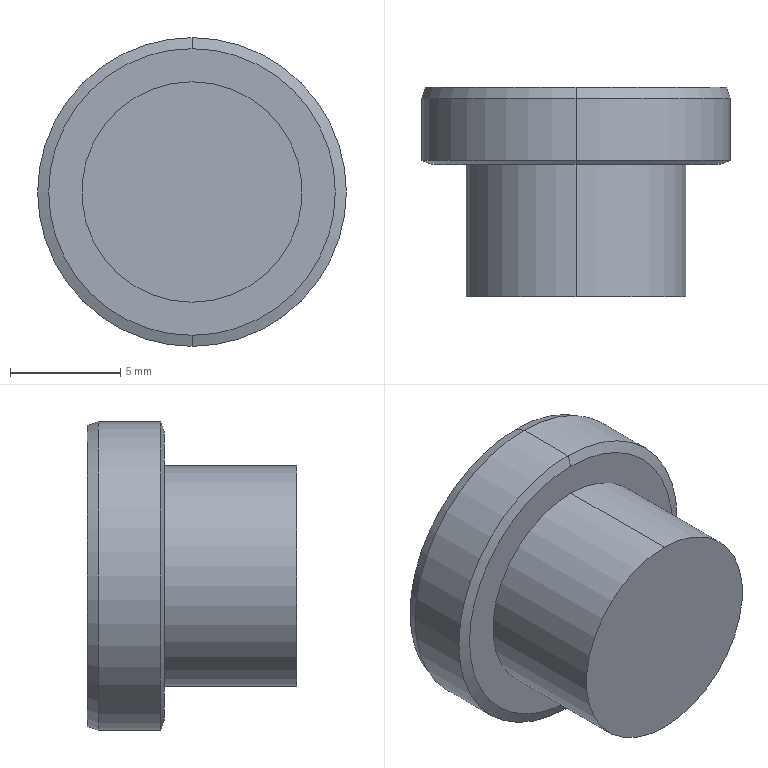Part | SolidWorks | features ICE 2, Chamfer 1, Extrusion 1 | 1 solid | 18 faces | box 14 x 9.5 x 14 mm | volume 897.832 mm3 | plane 10 | cone 4 | cylinder 4 | commonest cylinder face diameters 10 x2 14 x2
STEP:
#1=CARTESIAN_POINT('',(0.,9.5,6.818));
#2=VERTEX_POINT('',#1);
#3=CARTESIAN_POINT('',(0.,9.5,-6.818));
#4=VERTEX_POINT('',#3);
#5=CARTESIAN_POINT('',(0.,9.5,0.));
#6=DIRECTION('',(0.,1.,0.));
#7=DIRECTION('',(0.,0.,1.));
#8=AXIS2_PLACEMENT_3D('',#5,#6,#7);
#9=CIRCLE('',#8,6.818);
#10=EDGE_CURVE('',#2,#4,#9,.T.);
#11=ORIENTED_EDGE('',*,*,#10,.F.);
#12=CARTESIAN_POINT('',(0.,9.,7.));
#13=VERTEX_POINT('',#12);
#14=CARTESIAN_POINT('',(0.,9.5,6.818));
#15=DIRECTION('',(0.,-0.9397,0.342));
#16=VECTOR('',#15,1000.);
#17=LINE('',#14,#16);
#18=EDGE_CURVE('',#2,#13,#17,.T.);
#19=ORIENTED_EDGE('',*,*,#18,.T.);
#20=CARTESIAN_POINT('',(0.,9.,-7.));
#21=VERTEX_POINT('',#20);
#22=CARTESIAN_POINT('',(0.,9.,0.));
#23=DIRECTION('',(0.,-1.,0.));
#24=DIRECTION('',(0.,0.,1.));
#25=AXIS2_PLACEMENT_3D('',#22,#23,#24);
#26=CIRCLE('',#25,7.);
#27=EDGE_CURVE('',#21,#13,#26,.T.);
#28=ORIENTED_EDGE('',*,*,#27,.F.);
#29=CARTESIAN_POINT('',(0.,9.5,-6.818));
#30=DIRECTION('',(0.,-0.9397,-0.342));
#31=VECTOR('',#30,1000.);
#32=LINE('',#29,#31);
#33=EDGE_CURVE('',#4,#21,#32,.T.);
#34=ORIENTED_EDGE('',*,*,#33,.F.);
#35=EDGE_LOOP('',(#11,#19,#28,#34));
#36=FACE_OUTER_BOUND('',#35,.T.);
#37=CARTESIAN_POINT('',(0.,9.5,0.));
#38=DIRECTION('',(0.,-1.,0.));
#39=DIRECTION('',(0.,0.,-1.));
#40=AXIS2_PLACEMENT_3D('',#37,#38,#39);
#41=CONICAL_SURFACE('',#40,6.818,0.3491);
#42=ADVANCED_FACE('',(#36),#41,.T.);
#43=CARTESIAN_POINT('',(0.,6.,-6.5));
#44=VERTEX_POINT('',#43);
#45=CARTESIAN_POINT('',(0.,6.,6.5));
#46=VERTEX_POINT('',#45);
#47=CARTESIAN_POINT('',(0.,6.,0.));
#48=DIRECTION('',(0.,-1.,0.));
#49=DIRECTION('',(0.,0.,1.));
#50=AXIS2_PLACEMENT_3D('',#47,#48,#49);
#51=CIRCLE('',#50,6.5);
#52=EDGE_CURVE('',#44,#46,#51,.T.);
#53=ORIENTED_EDGE('',*,*,#52,.F.);
#54=CARTESIAN_POINT('',(0.,6.182,-7.));
#55=VERTEX_POINT('',#54);
#56=CARTESIAN_POINT('',(0.,6.182,-7.));
#57=DIRECTION('',(0.,0.342,-0.9397));
#58=VECTOR('',#57,1000.);
#59=LINE('',#56,#58);
#60=EDGE_CURVE('',#44,#55,#59,.T.);
#61=ORIENTED_EDGE('',*,*,#60,.T.);
#62=CARTESIAN_POINT('',(0.,6.182,7.));
#63=VERTEX_POINT('',#62);
#64=CARTESIAN_POINT('',(0.,6.182,0.));
#65=DIRECTION('',(0.,1.,0.));
#66=DIRECTION('',(0.,0.,1.));
#67=AXIS2_PLACEMENT_3D('',#64,#65,#66);
#68=CIRCLE('',#67,7.);
#69=EDGE_CURVE('',#63,#55,#68,.T.);
#70=ORIENTED_EDGE('',*,*,#69,.F.);
#71=CARTESIAN_POINT('',(0.,6.182,7.));
#72=DIRECTION('',(0.,0.342,0.9397));
#73=VECTOR('',#72,1000.);
#74=LINE('',#71,#73);
#75=EDGE_CURVE('',#46,#63,#74,.T.);
#76=ORIENTED_EDGE('',*,*,#75,.F.);
#77=EDGE_LOOP('',(#53,#61,#70,#76));
#78=FACE_OUTER_BOUND('',#77,.T.);
#79=CARTESIAN_POINT('',(0.,6.182,0.));
#80=DIRECTION('',(0.,1.,0.));
#81=DIRECTION('',(0.,0.,1.));
#82=AXIS2_PLACEMENT_3D('',#79,#80,#81);
#83=CONICAL_SURFACE('',#82,7.,1.222);
#84=ADVANCED_FACE('',(#78),#83,.T.);
#85=ORIENTED_EDGE('',*,*,#27,.T.);
#86=CARTESIAN_POINT('',(0.,9.5,7.));
#87=DIRECTION('',(0.,-1.,0.));
#88=VECTOR('',#87,1000.);
#89=LINE('',#86,#88);
#90=EDGE_CURVE('',#13,#63,#89,.T.);
#91=ORIENTED_EDGE('',*,*,#90,.T.);
#92=ORIENTED_EDGE('',*,*,#69,.T.);
#93=CARTESIAN_POINT('',(0.,9.5,-7.));
#94=DIRECTION('',(0.,-1.,0.));
#95=VECTOR('',#94,1000.);
#96=LINE('',#93,#95);
#97=EDGE_CURVE('',#21,#55,#96,.T.);
#98=ORIENTED_EDGE('',*,*,#97,.F.);
#99=EDGE_LOOP('',(#85,#91,#92,#98));
#100=FACE_OUTER_BOUND('',#99,.T.);
#101=CARTESIAN_POINT('',(0.,9.5,0.));
#102=DIRECTION('',(0.,-1.,0.));
#103=DIRECTION('',(0.,0.,-1.));
#104=AXIS2_PLACEMENT_3D('',#101,#102,#103);
#105=CYLINDRICAL_SURFACE('',#104,7.);
#106=ADVANCED_FACE('',(#100),#105,.T.);
#107=CARTESIAN_POINT('',(0.,6.,5.));
#108=VERTEX_POINT('',#107);
#109=CARTESIAN_POINT('',(0.,6.,-5.));
#110=VERTEX_POINT('',#109);
#111=CARTESIAN_POINT('',(0.,6.,0.));
#112=DIRECTION('',(0.,1.,0.));
#113=DIRECTION('',(0.,0.,1.));
#114=AXIS2_PLACEMENT_3D('',#111,#112,#113);
#115=CIRCLE('',#114,5.);
#116=EDGE_CURVE('',#108,#110,#115,.T.);
#117=ORIENTED_EDGE('',*,*,#116,.F.);
#118=CARTESIAN_POINT('',(0.,0.,5.));
#119=VERTEX_POINT('',#118);
#120=CARTESIAN_POINT('',(0.,6.,5.));
#121=DIRECTION('',(0.,-1.,0.));
#122=VECTOR('',#121,1000.);
#123=LINE('',#120,#122);
#124=EDGE_CURVE('',#108,#119,#123,.T.);
#125=ORIENTED_EDGE('',*,*,#124,.T.);
#126=CARTESIAN_POINT('',(0.,0.,-5.));
#127=VERTEX_POINT('',#126);
#128=CARTESIAN_POINT('',(0.,0.,0.));
#129=DIRECTION('',(0.,1.,0.));
#130=DIRECTION('',(0.,0.,1.));
#131=AXIS2_PLACEMENT_3D('',#128,#129,#130);
#132=CIRCLE('',#131,5.);
#133=EDGE_CURVE('',#119,#127,#132,.T.);
#134=ORIENTED_EDGE('',*,*,#133,.T.);
#135=CARTESIAN_POINT('',(0.,6.,-5.));
#136=DIRECTION('',(0.,-1.,0.));
#137=VECTOR('',#136,1000.);
#138=LINE('',#135,#137);
#139=EDGE_CURVE('',#110,#127,#138,.T.);
#140=ORIENTED_EDGE('',*,*,#139,.F.);
#141=EDGE_LOOP('',(#117,#125,#134,#140));
#142=FACE_OUTER_BOUND('',#141,.T.);
#143=CARTESIAN_POINT('',(0.,6.,0.));
#144=DIRECTION('',(0.,-1.,0.));
#145=DIRECTION('',(0.,0.,-1.));
#146=AXIS2_PLACEMENT_3D('',#143,#144,#145);
#147=CYLINDRICAL_SURFACE('',#146,5.);
#148=ADVANCED_FACE('',(#142),#147,.T.);
#149=ORIENTED_EDGE('',*,*,#124,.F.);
#150=CARTESIAN_POINT('',(0.,6.,0.));
#151=DIRECTION('',(0.,1.,0.));
#152=DIRECTION('',(0.,0.,1.));
#153=AXIS2_PLACEMENT_3D('',#150,#151,#152);
#154=CIRCLE('',#153,5.);
#155=EDGE_CURVE('',#110,#108,#154,.T.);
#156=ORIENTED_EDGE('',*,*,#155,.F.);
#157=ORIENTED_EDGE('',*,*,#139,.T.);
#158=CARTESIAN_POINT('',(0.,0.,0.));
#159=DIRECTION('',(0.,1.,0.));
#160=DIRECTION('',(0.,0.,1.));
#161=AXIS2_PLACEMENT_3D('',#158,#159,#160);
#162=CIRCLE('',#161,5.);
#163=EDGE_CURVE('',#127,#119,#162,.T.);
#164=ORIENTED_EDGE('',*,*,#163,.T.);
#165=EDGE_LOOP('',(#149,#156,#157,#164));
#166=FACE_OUTER_BOUND('',#165,.T.);
#167=CARTESIAN_POINT('',(0.,6.,0.));
#168=DIRECTION('',(0.,-1.,0.));
#169=DIRECTION('',(0.,0.,-1.));
#170=AXIS2_PLACEMENT_3D('',#167,#168,#169);
#171=CYLINDRICAL_SURFACE('',#170,5.);
#172=ADVANCED_FACE('',(#166),#171,.T.);
#173=ORIENTED_EDGE('',*,*,#163,.F.);
#174=ORIENTED_EDGE('',*,*,#133,.F.);
#175=EDGE_LOOP('',(#173,#174));
#176=FACE_OUTER_BOUND('',#175,.T.);
#177=CARTESIAN_POINT('',(0.,0.,0.));
#178=DIRECTION('',(0.,1.,0.));
#179=DIRECTION('',(0.,0.,1.));
#180=AXIS2_PLACEMENT_3D('',#177,#178,#179);
#181=PLANE('',#180);
#182=ADVANCED_FACE('',(#176),#181,.F.);
#183=ORIENTED_EDGE('',*,*,#90,.F.);
#184=CARTESIAN_POINT('',(0.,9.,0.));
#185=DIRECTION('',(0.,-1.,0.));
#186=DIRECTION('',(0.,0.,1.));
#187=AXIS2_PLACEMENT_3D('',#184,#185,#186);
#188=CIRCLE('',#187,7.);
#189=EDGE_CURVE('',#13,#21,#188,.T.);
#190=ORIENTED_EDGE('',*,*,#189,.T.);
#191=ORIENTED_EDGE('',*,*,#97,.T.);
#192=CARTESIAN_POINT('',(0.,6.182,0.));
#193=DIRECTION('',(0.,1.,0.));
#194=DIRECTION('',(0.,0.,1.));
#195=AXIS2_PLACEMENT_3D('',#192,#193,#194);
#196=CIRCLE('',#195,7.);
#197=EDGE_CURVE('',#55,#63,#196,.T.);
#198=ORIENTED_EDGE('',*,*,#197,.T.);
#199=EDGE_LOOP('',(#183,#190,#191,#198));
#200=FACE_OUTER_BOUND('',#199,.T.);
#201=CARTESIAN_POINT('',(0.,9.5,0.));
#202=DIRECTION('',(0.,-1.,0.));
#203=DIRECTION('',(0.,0.,-1.));
#204=AXIS2_PLACEMENT_3D('',#201,#202,#203);
#205=CYLINDRICAL_SURFACE('',#204,7.);
#206=ADVANCED_FACE('',(#200),#205,.T.);
#207=CARTESIAN_POINT('',(0.,9.5,0.));
#208=DIRECTION('',(0.,1.,0.));
#209=DIRECTION('',(0.,0.,1.));
#210=AXIS2_PLACEMENT_3D('',#207,#208,#209);
#211=CIRCLE('',#210,6.818);
#212=EDGE_CURVE('',#4,#2,#211,.T.);
#213=ORIENTED_EDGE('',*,*,#212,.T.);
#214=ORIENTED_EDGE('',*,*,#10,.T.);
#215=EDGE_LOOP('',(#213,#214));
#216=FACE_OUTER_BOUND('',#215,.T.);
#217=CARTESIAN_POINT('',(-1.443,9.5,-2.5));
#218=VERTEX_POINT('',#217);
#219=CARTESIAN_POINT('',(-2.887,9.5,0.));
#220=VERTEX_POINT('',#219);
#221=CARTESIAN_POINT('',(-1.443,9.5,-2.5));
#222=DIRECTION('',(-0.5,0.,0.866));
#223=VECTOR('',#222,1000.);
#224=LINE('',#221,#223);
#225=EDGE_CURVE('',#218,#220,#224,.T.);
#226=ORIENTED_EDGE('',*,*,#225,.F.);
#227=CARTESIAN_POINT('',(1.443,9.5,-2.5));
#228=VERTEX_POINT('',#227);
#229=CARTESIAN_POINT('',(1.443,9.5,-2.5));
#230=DIRECTION('',(-1.,0.,0.));
#231=VECTOR('',#230,1000.);
#232=LINE('',#229,#231);
#233=EDGE_CURVE('',#228,#218,#232,.T.);
#234=ORIENTED_EDGE('',*,*,#233,.F.);
#235=CARTESIAN_POINT('',(2.887,9.5,0.));
#236=VERTEX_POINT('',#235);
#237=CARTESIAN_POINT('',(2.887,9.5,0.));
#238=DIRECTION('',(-0.5,0.,-0.866));
#239=VECTOR('',#238,1000.);
#240=LINE('',#237,#239);
#241=EDGE_CURVE('',#236,#228,#240,.T.);
#242=ORIENTED_EDGE('',*,*,#241,.F.);
#243=CARTESIAN_POINT('',(1.443,9.5,2.5));
#244=VERTEX_POINT('',#243);
#245=CARTESIAN_POINT('',(1.443,9.5,2.5));
#246=DIRECTION('',(0.5,0.,-0.866));
#247=VECTOR('',#246,1000.);
#248=LINE('',#245,#247);
#249=EDGE_CURVE('',#244,#236,#248,.T.);
#250=ORIENTED_EDGE('',*,*,#249,.F.);
#251=CARTESIAN_POINT('',(-1.443,9.5,2.5));
#252=VERTEX_POINT('',#251);
#253=CARTESIAN_POINT('',(-1.443,9.5,2.5));
#254=DIRECTION('',(1.,0.,0.));
#255=VECTOR('',#254,1000.);
#256=LINE('',#253,#255);
#257=EDGE_CURVE('',#252,#244,#256,.T.);
#258=ORIENTED_EDGE('',*,*,#257,.F.);
#259=CARTESIAN_POINT('',(-2.887,9.5,0.));
#260=DIRECTION('',(0.5,0.,0.866));
#261=VECTOR('',#260,1000.);
#262=LINE('',#259,#261);
#263=EDGE_CURVE('',#220,#252,#262,.T.);
#264=ORIENTED_EDGE('',*,*,#263,.F.);
#265=EDGE_LOOP('',(#226,#234,#242,#250,#258,#264));
#266=FACE_BOUND('',#265,.T.);
#267=CARTESIAN_POINT('',(0.,9.5,0.));
#268=DIRECTION('',(0.,1.,0.));
#269=DIRECTION('',(0.,0.,1.));
#270=AXIS2_PLACEMENT_3D('',#267,#268,#269);
#271=PLANE('',#270);
#272=ADVANCED_FACE('',(#216,#266),#271,.T.);
#273=CARTESIAN_POINT('',(0.,6.,0.));
#274=DIRECTION('',(0.,-1.,0.));
#275=DIRECTION('',(0.,0.,1.));
#276=AXIS2_PLACEMENT_3D('',#273,#274,#275);
#277=CIRCLE('',#276,6.5);
#278=EDGE_CURVE('',#46,#44,#277,.T.);
#279=ORIENTED_EDGE('',*,*,#278,.T.);
#280=ORIENTED_EDGE('',*,*,#52,.T.);
#281=EDGE_LOOP('',(#279,#280));
#282=FACE_OUTER_BOUND('',#281,.T.);
#283=ORIENTED_EDGE('',*,*,#155,.T.);
#284=ORIENTED_EDGE('',*,*,#116,.T.);
#285=EDGE_LOOP('',(#283,#284));
#286=FACE_BOUND('',#285,.T.);
#287=CARTESIAN_POINT('',(0.,6.,0.));
#288=DIRECTION('',(0.,1.,0.));
#289=DIRECTION('',(0.,0.,1.));
#290=AXIS2_PLACEMENT_3D('',#287,#288,#289);
#291=PLANE('',#290);
#292=ADVANCED_FACE('',(#282,#286),#291,.F.);
#293=ORIENTED_EDGE('',*,*,#225,.T.);
#294=CARTESIAN_POINT('',(-2.887,4.5,0.));
#295=VERTEX_POINT('',#294);
#296=CARTESIAN_POINT('',(-2.887,4.5,0.));
#297=DIRECTION('',(0.,1.,0.));
#298=VECTOR('',#297,1000.);
#299=LINE('',#296,#298);
#300=EDGE_CURVE('',#295,#220,#299,.T.);
#301=ORIENTED_EDGE('',*,*,#300,.F.);
#302=CARTESIAN_POINT('',(-1.443,4.5,-2.5));
#303=VERTEX_POINT('',#302);
#304=CARTESIAN_POINT('',(-1.443,4.5,-2.5));
#305=DIRECTION('',(-0.5,0.,0.866));
#306=VECTOR('',#305,1000.);
#307=LINE('',#304,#306);
#308=EDGE_CURVE('',#303,#295,#307,.T.);
#309=ORIENTED_EDGE('',*,*,#308,.F.);
#310=CARTESIAN_POINT('',(-1.443,4.5,-2.5));
#311=DIRECTION('',(0.,1.,0.));
#312=VECTOR('',#311,1000.);
#313=LINE('',#310,#312);
#314=EDGE_CURVE('',#303,#218,#313,.T.);
#315=ORIENTED_EDGE('',*,*,#314,.T.);
#316=EDGE_LOOP('',(#293,#301,#309,#315));
#317=FACE_OUTER_BOUND('',#316,.T.);
#318=CARTESIAN_POINT('',(-1.443,4.5,-2.5));
#319=DIRECTION('',(-0.866,0.,-0.5));
#320=DIRECTION('',(-0.5,0.,0.866));
#321=AXIS2_PLACEMENT_3D('',#318,#319,#320);
#322=PLANE('',#321);
#323=ADVANCED_FACE('',(#317),#322,.F.);
#324=ORIENTED_EDGE('',*,*,#233,.T.);
#325=ORIENTED_EDGE('',*,*,#314,.F.);
#326=CARTESIAN_POINT('',(1.443,4.5,-2.5));
#327=VERTEX_POINT('',#326);
#328=CARTESIAN_POINT('',(1.443,4.5,-2.5));
#329=DIRECTION('',(-1.,0.,0.));
#330=VECTOR('',#329,1000.);
#331=LINE('',#328,#330);
#332=EDGE_CURVE('',#327,#303,#331,.T.);
#333=ORIENTED_EDGE('',*,*,#332,.F.);
#334=CARTESIAN_POINT('',(1.443,4.5,-2.5));
#335=DIRECTION('',(0.,1.,0.));
#336=VECTOR('',#335,1000.);
#337=LINE('',#334,#336);
#338=EDGE_CURVE('',#327,#228,#337,.T.);
#339=ORIENTED_EDGE('',*,*,#338,.T.);
#340=EDGE_LOOP('',(#324,#325,#333,#339));
#341=FACE_OUTER_BOUND('',#340,.T.);
#342=CARTESIAN_POINT('',(1.443,4.5,-2.5));
#343=DIRECTION('',(0.,0.,-1.));
#344=DIRECTION('',(-1.,0.,0.));
#345=AXIS2_PLACEMENT_3D('',#342,#343,#344);
#346=PLANE('',#345);
#347=ADVANCED_FACE('',(#341),#346,.F.);
#348=ORIENTED_EDGE('',*,*,#241,.T.);
#349=ORIENTED_EDGE('',*,*,#338,.F.);
#350=CARTESIAN_POINT('',(2.887,4.5,0.));
#351=VERTEX_POINT('',#350);
#352=CARTESIAN_POINT('',(2.887,4.5,0.));
#353=DIRECTION('',(-0.5,0.,-0.866));
#354=VECTOR('',#353,1000.);
#355=LINE('',#352,#354);
#356=EDGE_CURVE('',#351,#327,#355,.T.);
#357=ORIENTED_EDGE('',*,*,#356,.F.);
#358=CARTESIAN_POINT('',(2.887,4.5,0.));
#359=DIRECTION('',(0.,1.,0.));
#360=VECTOR('',#359,1000.);
#361=LINE('',#358,#360);
#362=EDGE_CURVE('',#351,#236,#361,.T.);
#363=ORIENTED_EDGE('',*,*,#362,.T.);
#364=EDGE_LOOP('',(#348,#349,#357,#363));
#365=FACE_OUTER_BOUND('',#364,.T.);
#366=CARTESIAN_POINT('',(2.887,4.5,0.));
#367=DIRECTION('',(0.866,0.,-0.5));
#368=DIRECTION('',(-0.5,0.,-0.866));
#369=AXIS2_PLACEMENT_3D('',#366,#367,#368);
#370=PLANE('',#369);
#371=ADVANCED_FACE('',(#365),#370,.F.);
#372=ORIENTED_EDGE('',*,*,#249,.T.);
#373=ORIENTED_EDGE('',*,*,#362,.F.);
#374=CARTESIAN_POINT('',(1.443,4.5,2.5));
#375=VERTEX_POINT('',#374);
#376=CARTESIAN_POINT('',(1.443,4.5,2.5));
#377=DIRECTION('',(0.5,0.,-0.866));
#378=VECTOR('',#377,1000.);
#379=LINE('',#376,#378);
#380=EDGE_CURVE('',#375,#351,#379,.T.);
#381=ORIENTED_EDGE('',*,*,#380,.F.);
#382=CARTESIAN_POINT('',(1.443,4.5,2.5));
#383=DIRECTION('',(0.,1.,0.));
#384=VECTOR('',#383,1000.);
#385=LINE('',#382,#384);
#386=EDGE_CURVE('',#375,#244,#385,.T.);
#387=ORIENTED_EDGE('',*,*,#386,.T.);
#388=EDGE_LOOP('',(#372,#373,#381,#387));
#389=FACE_OUTER_BOUND('',#388,.T.);
#390=CARTESIAN_POINT('',(1.443,4.5,2.5));
#391=DIRECTION('',(0.866,0.,0.5));
#392=DIRECTION('',(0.5,0.,-0.866));
#393=AXIS2_PLACEMENT_3D('',#390,#391,#392);
#394=PLANE('',#393);
#395=ADVANCED_FACE('',(#389),#394,.F.);
#396=ORIENTED_EDGE('',*,*,#257,.T.);
#397=ORIENTED_EDGE('',*,*,#386,.F.);
#398=CARTESIAN_POINT('',(-1.443,4.5,2.5));
#399=VERTEX_POINT('',#398);
#400=CARTESIAN_POINT('',(-1.443,4.5,2.5));
#401=DIRECTION('',(1.,0.,0.));
#402=VECTOR('',#401,1000.);
#403=LINE('',#400,#402);
#404=EDGE_CURVE('',#399,#375,#403,.T.);
#405=ORIENTED_EDGE('',*,*,#404,.F.);
#406=CARTESIAN_POINT('',(-1.443,4.5,2.5));
#407=DIRECTION('',(0.,1.,0.));
#408=VECTOR('',#407,1000.);
#409=LINE('',#406,#408);
#410=EDGE_CURVE('',#399,#252,#409,.T.);
#411=ORIENTED_EDGE('',*,*,#410,.T.);
#412=EDGE_LOOP('',(#396,#397,#405,#411));
#413=FACE_OUTER_BOUND('',#412,.T.);
#414=CARTESIAN_POINT('',(-1.443,4.5,2.5));
#415=DIRECTION('',(0.,0.,1.));
#416=DIRECTION('',(1.,0.,0.));
#417=AXIS2_PLACEMENT_3D('',#414,#415,#416);
#418=PLANE('',#417);
#419=ADVANCED_FACE('',(#413),#418,.F.);
#420=ORIENTED_EDGE('',*,*,#263,.T.);
#421=ORIENTED_EDGE('',*,*,#410,.F.);
#422=CARTESIAN_POINT('',(-2.887,4.5,0.));
#423=DIRECTION('',(0.5,0.,0.866));
#424=VECTOR('',#423,1000.);
#425=LINE('',#422,#424);
#426=EDGE_CURVE('',#295,#399,#425,.T.);
#427=ORIENTED_EDGE('',*,*,#426,.F.);
#428=ORIENTED_EDGE('',*,*,#300,.T.);
#429=EDGE_LOOP('',(#420,#421,#427,#428));
#430=FACE_OUTER_BOUND('',#429,.T.);
#431=CARTESIAN_POINT('',(-2.887,4.5,0.));
#432=DIRECTION('',(-0.866,0.,0.5));
#433=DIRECTION('',(0.5,0.,0.866));
#434=AXIS2_PLACEMENT_3D('',#431,#432,#433);
#435=PLANE('',#434);
#436=ADVANCED_FACE('',(#430),#435,.F.);
#437=ORIENTED_EDGE('',*,*,#308,.T.);
#438=ORIENTED_EDGE('',*,*,#426,.T.);
#439=ORIENTED_EDGE('',*,*,#404,.T.);
#440=ORIENTED_EDGE('',*,*,#380,.T.);
#441=ORIENTED_EDGE('',*,*,#356,.T.);
#442=ORIENTED_EDGE('',*,*,#332,.T.);
#443=EDGE_LOOP('',(#437,#438,#439,#440,#441,#442));
#444=FACE_OUTER_BOUND('',#443,.T.);
#445=CARTESIAN_POINT('',(0.,4.5,0.));
#446=DIRECTION('',(0.,1.,0.));
#447=DIRECTION('',(0.,0.,1.));
#448=AXIS2_PLACEMENT_3D('',#445,#446,#447);
#449=PLANE('',#448);
#450=ADVANCED_FACE('',(#444),#449,.T.);
#451=ORIENTED_EDGE('',*,*,#60,.F.);
#452=ORIENTED_EDGE('',*,*,#278,.F.);
#453=ORIENTED_EDGE('',*,*,#75,.T.);
#454=ORIENTED_EDGE('',*,*,#197,.F.);
#455=EDGE_LOOP('',(#451,#452,#453,#454));
#456=FACE_OUTER_BOUND('',#455,.T.);
#457=CARTESIAN_POINT('',(0.,6.182,0.));
#458=DIRECTION('',(0.,1.,0.));
#459=DIRECTION('',(0.,0.,1.));
#460=AXIS2_PLACEMENT_3D('',#457,#458,#459);
#461=CONICAL_SURFACE('',#460,7.,1.222);
#462=ADVANCED_FACE('',(#456),#461,.T.);
#463=ORIENTED_EDGE('',*,*,#18,.F.);
#464=ORIENTED_EDGE('',*,*,#212,.F.);
#465=ORIENTED_EDGE('',*,*,#33,.T.);
#466=ORIENTED_EDGE('',*,*,#189,.F.);
#467=EDGE_LOOP('',(#463,#464,#465,#466));
#468=FACE_OUTER_BOUND('',#467,.T.);
#469=CARTESIAN_POINT('',(0.,9.5,0.));
#470=DIRECTION('',(0.,-1.,0.));
#471=DIRECTION('',(0.,0.,-1.));
#472=AXIS2_PLACEMENT_3D('',#469,#470,#471);
#473=CONICAL_SURFACE('',#472,6.818,0.3491);
#474=ADVANCED_FACE('',(#468),#473,.T.);
#475=CLOSED_SHELL('',(#42,#84,#106,#148,#172,#182,#206,#272,#292,#323,#347,#371,#395,#419,#436,#450,#462,#474));
#476=MANIFOLD_SOLID_BREP('',#475);
#477=CARTESIAN_POINT('',(0.,0.,0.));
#478=DIRECTION('',(0.,0.,1.));
#479=DIRECTION('',(1.,0.,0.));
#480=AXIS2_PLACEMENT_3D('',#477,#478,#479);
#481=(LENGTH_UNIT()NAMED_UNIT(*)SI_UNIT(.MILLI.,.METRE.));
#482=UNCERTAINTY_MEASURE_WITH_UNIT(LENGTH_MEASURE(0.00001),#481,'','');
#483=(NAMED_UNIT(*)PLANE_ANGLE_UNIT()SI_UNIT($,.RADIAN.));
#484=(NAMED_UNIT(*)SI_UNIT($,.STERADIAN.)SOLID_ANGLE_UNIT());
#485=(GEOMETRIC_REPRESENTATION_CONTEXT(3)GLOBAL_UNCERTAINTY_ASSIGNED_CONTEXT((#482))GLOBAL_UNIT_ASSIGNED_CONTEXT((#481,#483,#484))REPRESENTATION_CONTEXT('',''));
#486=ADVANCED_BREP_SHAPE_REPRESENTATION('',(#476,#480),#485);